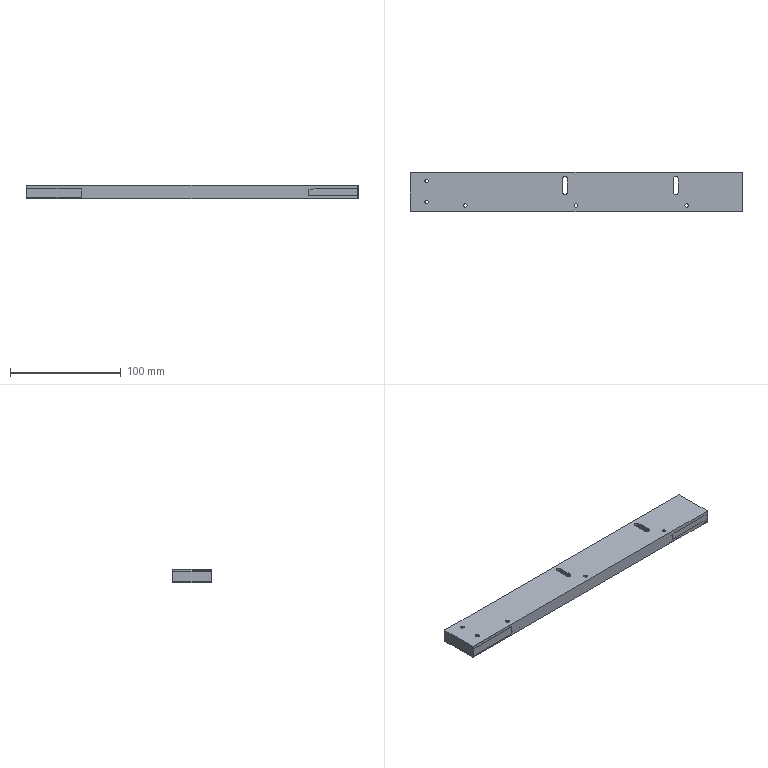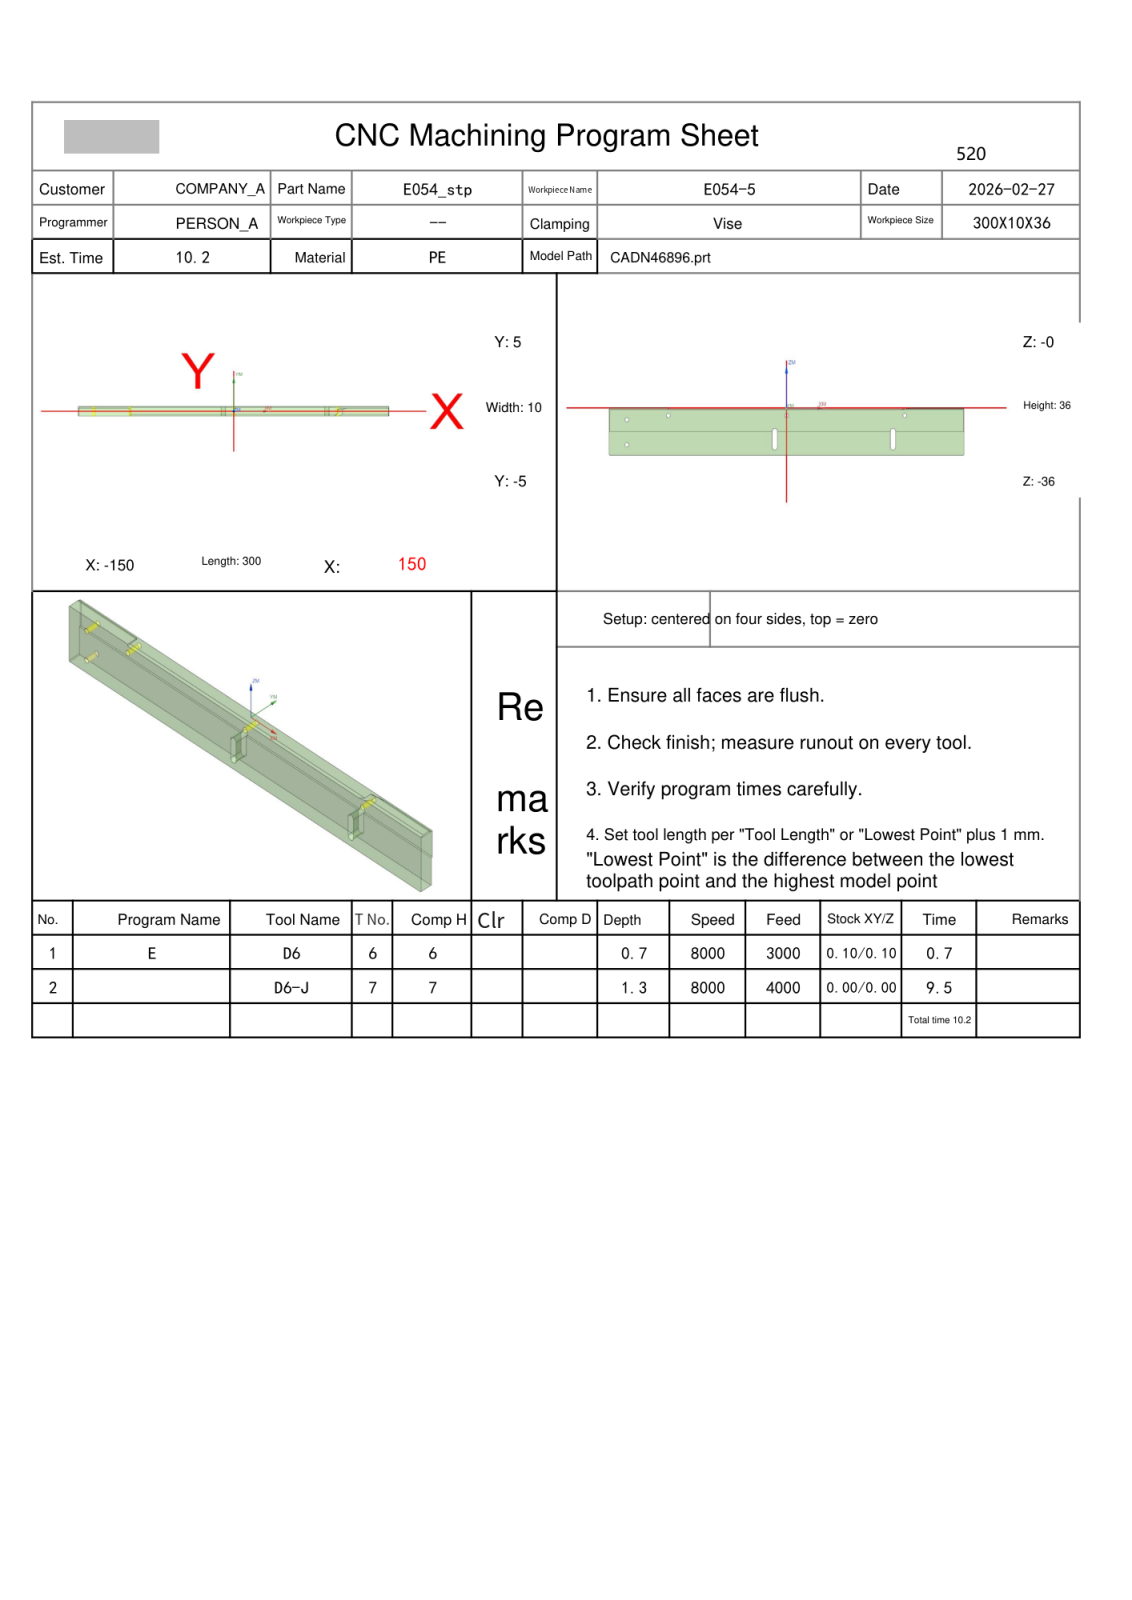NC program | NX | posted by the shop | part box 300 x 36 x 12 mm
Lines 1 to 116 of 2760:
%
O0001
(Machine time: 10.64 MIN)
(===Total Tool:2===)
(T6=D6      D=6.   R=0.   D-  H06 Z=-0.7  )
(T7=D6-J    D=6.   R=0.   D7  H07 Z=-1.3  )
G80 G90 G17 G49 G40
G91 G28 Z0
M01
N1 T06 M06
(D6  D=6. R=0. H=06 ce=0.10 di=0.10)
G00 G90 G54 X.312 Y10.5 M03 S8000
G43 H06 Z10.1
M08
Z1.15
G01 Z-.35 F3000.
Y7.44
X152.94
Y5.9
X106.937
G03 X106.492 Y5.903 I-.446 J-30.538
X102.043 Y5.577 I0.0 J-30.542
G01 X101.204 Y5.425
X100.402 Y5.221
X99.536 Y4.896
X98.314 Y4.102
X97.525 Y2.538
Y-5.94
X-96.9
Y5.9
X-152.94
Y7.44
X-1.508
G02 X-1.01 Y7.173 I-.001 J-.6
G01 X1.635 Y3.207
G03 X2.133 Y2.94 I.499 J.333
G01 X92.428
G02 X93.025 Y2.343 I-.003 J-.6
G01 Y-.843
G02 X92.428 Y-1.44 I-.6 J.003
G01 X-91.803
G02 X-92.4 Y-.843 I.003 J.6
G01 Y2.343
G02 X-91.803 Y2.94 I.6 J-.003
G01 X.312
X.812
Y10.5
Z1.15
G00 X.169
Z.8
G01 Z-.7
Y7.44
X152.94
Y5.9
X150.967
X150.764 Y5.964
X150.357 Y6.039
X106.456 Y6.04
X104.951 Y6.004
X103.442 Y5.911
X101.93 Y5.735
X99.935 Y5.347
X98.864 Y4.815
X98.589 Y4.641
X98.175 Y4.319
X97.456 Y3.563
X97.409 Y3.532
X97.408 Y3.476
X97.298 Y3.058
X97.136 Y2.777
X97.097 Y2.739
X97.108 Y2.686
X97.052 Y1.5
Y-4.478
X97.201 Y-5.94
X-96.868
X-96.786 Y-5.772
X-96.752 Y-5.736
X-96.766 Y-5.688
X-96.747 Y3.001
X-96.809 Y3.42
X-96.9 Y3.792
Y5.9
X-99.034
X-99.477 Y6.036
X-150.357 Y6.039
X-150.764 Y5.964
X-150.967 Y5.9
X-152.94
Y7.44
X-1.651
G02 X-1.153 Y7.173 I-.001 J-.6
G01 X1.492 Y3.207
G03 X1.99 Y2.94 I.499 J.333
G01 X91.989
G02 X92.586 Y2.34 I-.003 J-.6
G01 Y2.315
X92.552 Y1.608
Y-.843
G02 X91.955 Y-1.44 I-.6 J.003
G01 X-91.65
G02 X-92.247 Y-.843 I.003 J.6
G01 Y2.343
G02 X-91.65 Y2.94 I.6 J-.003
G01 X.169
X.669
Y10.5
Z.8
G00 Z10.1
G91 G28 Z0.0
M05
M09
G91 G28 Z0.0
M01